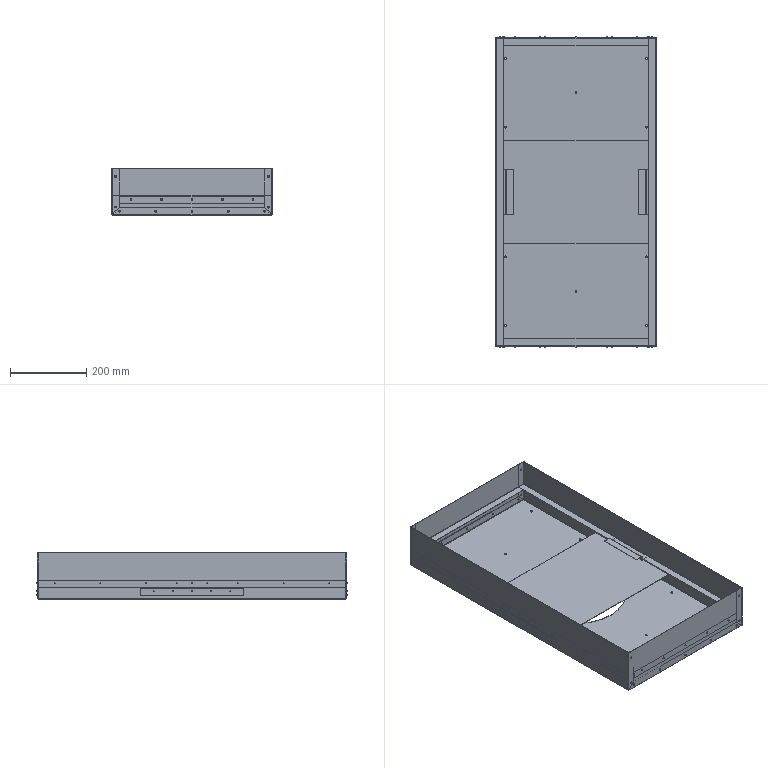Part | SolidWorks | features ReferencePattern 29, CompositeCurve 6, MirrorCompFeat 3 | 62 solids | 1130 faces | box 422.6 x 813.6 x 121 mm | volume 827585 mm3 | cylinder 614 | plane 388 | sphere 104 | cone 16 | spline 8 | commonest cylinder face diameters 2.4 x220 2.5 x208 2.65 x104 1.473 x20 5 x20 3.2 x16